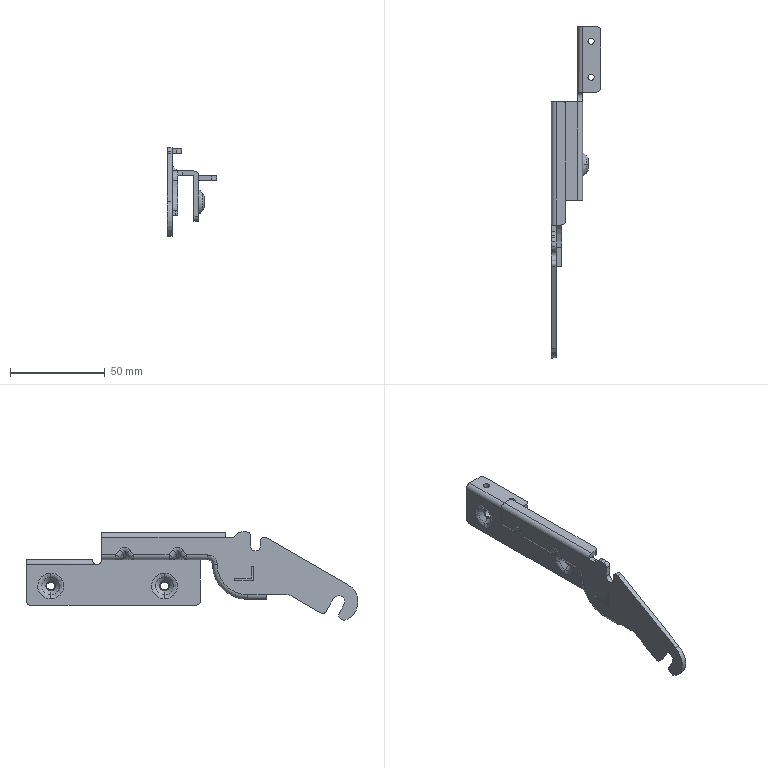Part | STEP file | ZXW722-L-31 | 1 solid | 147 faces | box 25.95 x 175.067 x 46.477 mm | volume 15631 mm3 | cylinder 58 | plane 51 | spline 36 | torus 2 | commonest cylinder face diameters 5 x15 6 x10 1 x8 2 x4 3.3 x4 4.2 x4